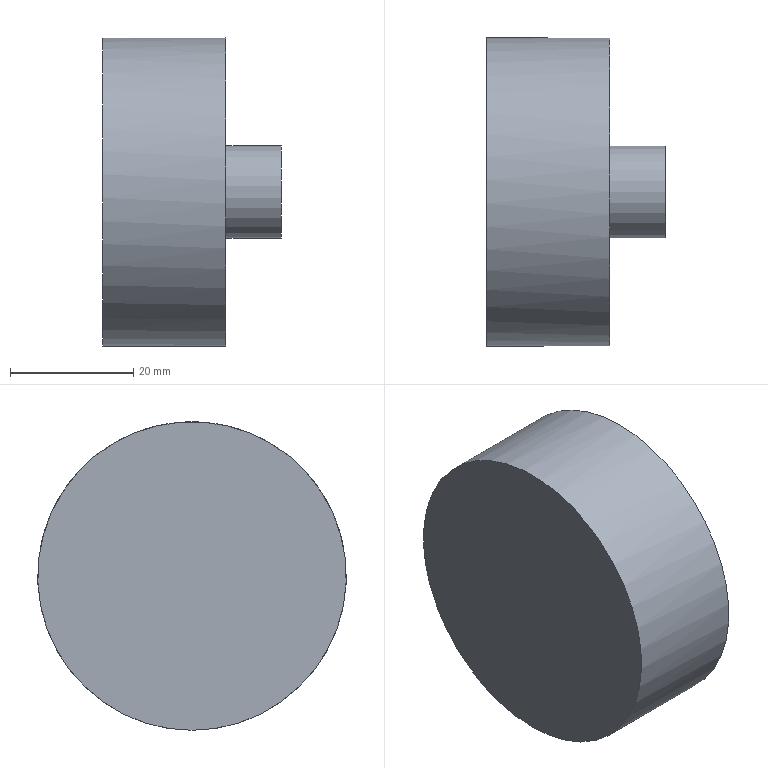Part | STEP file | Tube necking machine_id618_x_t | 1 solid | 5 faces | box 29 x 50 x 50 mm | volume 40860 mm3 | plane 3 | cylinder 2 | commonest cylinder face diameters 15 x1 50 x1
STEP:
#1=CARTESIAN_POINT('',(0.,0.,0.));
#2=DIRECTION('',(0.,0.,1.));
#3=DIRECTION('',(1.,0.,0.));
#4=AXIS2_PLACEMENT_3D('',#1,#2,#3);
#5=CARTESIAN_POINT('',(270.5,50.,197.5));
#6=VERTEX_POINT('',#5);
#7=CARTESIAN_POINT('',(270.5,50.,182.5));
#8=VERTEX_POINT('',#7);
#9=CARTESIAN_POINT('',(270.5,50.,190.));
#10=DIRECTION('',(1.,0.,0.));
#11=DIRECTION('',(0.,0.,1.));
#12=AXIS2_PLACEMENT_3D('',#9,#10,#11);
#13=CIRCLE('',#12,7.5);
#14=CARTESIAN_POINT('',(274.5,50.,190.));
#15=DIRECTION('',(1.,0.,0.));
#16=DIRECTION('',(0.,0.,-1.));
#17=AXIS2_PLACEMENT_3D('',#14,#15,#16);
#18=CYLINDRICAL_SURFACE('',#17,7.5);
#19=CARTESIAN_POINT('',(3.142,-4.));
#20=DIRECTION('',(1.,0.));
#21=VECTOR('',#20,1.);
#22=LINE('',#19,#21);
#23=(GEOMETRIC_REPRESENTATION_CONTEXT(2)PARAMETRIC_REPRESENTATION_CONTEXT()REPRESENTATION_CONTEXT('',''));
#24=DEFINITIONAL_REPRESENTATION('',(#22),#23);
#25=PCURVE('',#18,#24);
#26=CARTESIAN_POINT('',(270.5,50.,190.));
#27=DIRECTION('',(-1.,0.,0.));
#28=DIRECTION('',(0.,0.,1.));
#29=AXIS2_PLACEMENT_3D('',#26,#27,#28);
#30=PLANE('',#29);
#31=CARTESIAN_POINT('',(7.5,0.));
#32=CARTESIAN_POINT('',(7.5,-12.99));
#33=CARTESIAN_POINT('',(-3.75,-6.495));
#34=CARTESIAN_POINT('',(-15.,0.));
#35=CARTESIAN_POINT('',(-3.75,6.495));
#36=CARTESIAN_POINT('',(7.5,12.99));
#37=CARTESIAN_POINT('',(7.5,0.));
#38=(BOUNDED_CURVE()B_SPLINE_CURVE(2,(#31,#32,#33,#34,#35,#36,#37),.UNSPECIFIED.,.T.,.F.)B_SPLINE_CURVE_WITH_KNOTS((1,2,2,2,2,1),(-2.094,0.,2.094,4.189,6.283,8.378),.UNSPECIFIED.)CURVE()GEOMETRIC_REPRESENTATION_ITEM()RATIONAL_B_SPLINE_CURVE((1.,0.5,1.,0.5,1.,0.5,1.))REPRESENTATION_ITEM(''));
#39=(GEOMETRIC_REPRESENTATION_CONTEXT(2)PARAMETRIC_REPRESENTATION_CONTEXT()REPRESENTATION_CONTEXT('',''));
#40=DEFINITIONAL_REPRESENTATION('',(#38),#39);
#41=PCURVE('',#30,#40);
#42=SURFACE_CURVE('',#13,(#25,#41),.PCURVE_S1.);
#43=EDGE_CURVE('',#6,#8,#42,.T.);
#44=ORIENTED_EDGE('',*,*,#43,.T.);
#45=CARTESIAN_POINT('',(279.5,50.,182.5));
#46=VERTEX_POINT('',#45);
#47=CARTESIAN_POINT('',(270.5,50.,182.5));
#48=CARTESIAN_POINT('',(279.5,50.,182.5));
#49=B_SPLINE_CURVE_WITH_KNOTS('',1,(#47,#48),.UNSPECIFIED.,.F.,.F.,(2,2),(-4.,5.),.PIECEWISE_BEZIER_KNOTS.);
#50=CARTESIAN_POINT('',(6.283,0.));
#51=DIRECTION('',(0.,1.));
#52=VECTOR('',#51,1.);
#53=LINE('',#50,#52);
#54=(GEOMETRIC_REPRESENTATION_CONTEXT(2)PARAMETRIC_REPRESENTATION_CONTEXT()REPRESENTATION_CONTEXT('',''));
#55=DEFINITIONAL_REPRESENTATION('',(#53),#54);
#56=PCURVE('',#18,#55);
#57=CARTESIAN_POINT('',(0.,0.));
#58=DIRECTION('',(0.,1.));
#59=VECTOR('',#58,1.);
#60=LINE('',#57,#59);
#61=(GEOMETRIC_REPRESENTATION_CONTEXT(2)PARAMETRIC_REPRESENTATION_CONTEXT()REPRESENTATION_CONTEXT('',''));
#62=DEFINITIONAL_REPRESENTATION('',(#60),#61);
#63=PCURVE('',#18,#62);
#64=SEAM_CURVE('',#49,(#56,#63),.PCURVE_S1.);
#65=EDGE_CURVE('',#8,#46,#64,.T.);
#66=ORIENTED_EDGE('',*,*,#65,.T.);
#67=CARTESIAN_POINT('',(279.5,50.,190.));
#68=DIRECTION('',(1.,0.,0.));
#69=DIRECTION('',(0.,0.,-1.));
#70=AXIS2_PLACEMENT_3D('',#67,#68,#69);
#71=CIRCLE('',#70,7.5);
#72=CARTESIAN_POINT('',(0.,5.));
#73=DIRECTION('',(1.,0.));
#74=VECTOR('',#73,1.);
#75=LINE('',#72,#74);
#76=(GEOMETRIC_REPRESENTATION_CONTEXT(2)PARAMETRIC_REPRESENTATION_CONTEXT()REPRESENTATION_CONTEXT('',''));
#77=DEFINITIONAL_REPRESENTATION('',(#75),#76);
#78=PCURVE('',#18,#77);
#79=CARTESIAN_POINT('',(279.5,50.,190.));
#80=DIRECTION('',(1.,0.,0.));
#81=DIRECTION('',(0.,0.,-1.));
#82=AXIS2_PLACEMENT_3D('',#79,#80,#81);
#83=PLANE('',#82);
#84=CARTESIAN_POINT('',(0.,0.));
#85=DIRECTION('',(1.,0.));
#86=AXIS2_PLACEMENT_2D('',#84,#85);
#87=CIRCLE('',#86,7.5);
#88=(GEOMETRIC_REPRESENTATION_CONTEXT(2)PARAMETRIC_REPRESENTATION_CONTEXT()REPRESENTATION_CONTEXT('',''));
#89=DEFINITIONAL_REPRESENTATION('',(#87),#88);
#90=PCURVE('',#83,#89);
#91=SURFACE_CURVE('',#71,(#78,#90),.PCURVE_S1.);
#92=EDGE_CURVE('',#46,#46,#91,.T.);
#93=ORIENTED_EDGE('',*,*,#92,.F.);
#94=ORIENTED_EDGE('',*,*,#65,.F.);
#95=CARTESIAN_POINT('',(270.5,50.,190.));
#96=DIRECTION('',(1.,0.,0.));
#97=DIRECTION('',(0.,0.,1.));
#98=AXIS2_PLACEMENT_3D('',#95,#96,#97);
#99=CIRCLE('',#98,7.5);
#100=CARTESIAN_POINT('',(-3.142,-4.));
#101=DIRECTION('',(1.,0.));
#102=VECTOR('',#101,1.);
#103=LINE('',#100,#102);
#104=(GEOMETRIC_REPRESENTATION_CONTEXT(2)PARAMETRIC_REPRESENTATION_CONTEXT()REPRESENTATION_CONTEXT('',''));
#105=DEFINITIONAL_REPRESENTATION('',(#103),#104);
#106=PCURVE('',#18,#105);
#107=CARTESIAN_POINT('',(7.5,0.));
#108=CARTESIAN_POINT('',(7.5,-12.99));
#109=CARTESIAN_POINT('',(-3.75,-6.495));
#110=CARTESIAN_POINT('',(-15.,0.));
#111=CARTESIAN_POINT('',(-3.75,6.495));
#112=CARTESIAN_POINT('',(7.5,12.99));
#113=CARTESIAN_POINT('',(7.5,0.));
#114=(BOUNDED_CURVE()B_SPLINE_CURVE(2,(#107,#108,#109,#110,#111,#112,#113),.UNSPECIFIED.,.T.,.F.)B_SPLINE_CURVE_WITH_KNOTS((1,2,2,2,2,1),(-2.094,0.,2.094,4.189,6.283,8.378),.UNSPECIFIED.)CURVE()GEOMETRIC_REPRESENTATION_ITEM()RATIONAL_B_SPLINE_CURVE((1.,0.5,1.,0.5,1.,0.5,1.))REPRESENTATION_ITEM(''));
#115=(GEOMETRIC_REPRESENTATION_CONTEXT(2)PARAMETRIC_REPRESENTATION_CONTEXT()REPRESENTATION_CONTEXT('',''));
#116=DEFINITIONAL_REPRESENTATION('',(#114),#115);
#117=PCURVE('',#30,#116);
#118=SURFACE_CURVE('',#99,(#106,#117),.PCURVE_S1.);
#119=EDGE_CURVE('',#8,#6,#118,.T.);
#120=ORIENTED_EDGE('',*,*,#119,.T.);
#121=EDGE_LOOP('',(#44,#66,#93,#94,#120));
#122=FACE_BOUND('',#121,.T.);
#123=ADVANCED_FACE('',(#122),#18,.T.);
#124=ORIENTED_EDGE('',*,*,#92,.T.);
#125=EDGE_LOOP('',(#124));
#126=FACE_BOUND('',#125,.T.);
#127=ADVANCED_FACE('',(#126),#83,.T.);
#128=CARTESIAN_POINT('',(250.5,50.,165.));
#129=VERTEX_POINT('',#128);
#130=CARTESIAN_POINT('',(250.5,50.,190.));
#131=DIRECTION('',(1.,0.,0.));
#132=DIRECTION('',(0.,0.,-1.));
#133=AXIS2_PLACEMENT_3D('',#130,#131,#132);
#134=CIRCLE('',#133,25.);
#135=CARTESIAN_POINT('',(250.5,80.,332.));
#136=DIRECTION('',(1.,0.,0.));
#137=DIRECTION('',(0.,0.,-1.));
#138=AXIS2_PLACEMENT_3D('',#135,#136,#137);
#139=PLANE('',#138);
#140=CARTESIAN_POINT('',(142.,-30.));
#141=DIRECTION('',(1.,0.));
#142=AXIS2_PLACEMENT_2D('',#140,#141);
#143=CIRCLE('',#142,25.);
#144=(GEOMETRIC_REPRESENTATION_CONTEXT(2)PARAMETRIC_REPRESENTATION_CONTEXT()REPRESENTATION_CONTEXT('',''));
#145=DEFINITIONAL_REPRESENTATION('',(#143),#144);
#146=PCURVE('',#139,#145);
#147=CARTESIAN_POINT('',(36.9,50.,190.));
#148=DIRECTION('',(1.,0.,0.));
#149=DIRECTION('',(0.,0.,-1.));
#150=AXIS2_PLACEMENT_3D('',#147,#148,#149);
#151=CYLINDRICAL_SURFACE('',#150,25.);
#152=CARTESIAN_POINT('',(0.,213.6));
#153=DIRECTION('',(1.,0.));
#154=VECTOR('',#153,1.);
#155=LINE('',#152,#154);
#156=(GEOMETRIC_REPRESENTATION_CONTEXT(2)PARAMETRIC_REPRESENTATION_CONTEXT()REPRESENTATION_CONTEXT('',''));
#157=DEFINITIONAL_REPRESENTATION('',(#155),#156);
#158=PCURVE('',#151,#157);
#159=SURFACE_CURVE('',#134,(#146,#158),.PCURVE_S1.);
#160=EDGE_CURVE('',#129,#129,#159,.T.);
#161=ORIENTED_EDGE('',*,*,#160,.F.);
#162=EDGE_LOOP('',(#161));
#163=FACE_BOUND('',#162,.T.);
#164=ADVANCED_FACE('',(#163),#139,.F.);
#165=ORIENTED_EDGE('',*,*,#43,.F.);
#166=ORIENTED_EDGE('',*,*,#119,.F.);
#167=EDGE_LOOP('',(#165,#166));
#168=FACE_BOUND('',#167,.T.);
#169=CARTESIAN_POINT('',(270.5,50.,215.));
#170=VERTEX_POINT('',#169);
#171=CARTESIAN_POINT('',(270.5,50.,165.));
#172=VERTEX_POINT('',#171);
#173=CARTESIAN_POINT('',(270.5,50.,190.));
#174=DIRECTION('',(-1.,0.,0.));
#175=DIRECTION('',(0.,0.,1.));
#176=AXIS2_PLACEMENT_3D('',#173,#174,#175);
#177=CIRCLE('',#176,25.);
#178=CARTESIAN_POINT('',(0.,0.));
#179=DIRECTION('',(1.,0.));
#180=AXIS2_PLACEMENT_2D('',#178,#179);
#181=CIRCLE('',#180,25.);
#182=(GEOMETRIC_REPRESENTATION_CONTEXT(2)PARAMETRIC_REPRESENTATION_CONTEXT()REPRESENTATION_CONTEXT('',''));
#183=DEFINITIONAL_REPRESENTATION('',(#181),#182);
#184=PCURVE('',#30,#183);
#185=CARTESIAN_POINT('',(3.142,233.6));
#186=DIRECTION('',(-1.,0.));
#187=VECTOR('',#186,1.);
#188=LINE('',#185,#187);
#189=(GEOMETRIC_REPRESENTATION_CONTEXT(2)PARAMETRIC_REPRESENTATION_CONTEXT()REPRESENTATION_CONTEXT('',''));
#190=DEFINITIONAL_REPRESENTATION('',(#188),#189);
#191=PCURVE('',#151,#190);
#192=SURFACE_CURVE('',#177,(#184,#191),.PCURVE_S1.);
#193=EDGE_CURVE('',#170,#172,#192,.T.);
#194=ORIENTED_EDGE('',*,*,#193,.F.);
#195=CARTESIAN_POINT('',(270.5,50.,190.));
#196=DIRECTION('',(-1.,0.,0.));
#197=DIRECTION('',(0.,0.,1.));
#198=AXIS2_PLACEMENT_3D('',#195,#196,#197);
#199=CIRCLE('',#198,25.);
#200=CARTESIAN_POINT('',(0.,0.));
#201=DIRECTION('',(1.,0.));
#202=AXIS2_PLACEMENT_2D('',#200,#201);
#203=CIRCLE('',#202,25.);
#204=(GEOMETRIC_REPRESENTATION_CONTEXT(2)PARAMETRIC_REPRESENTATION_CONTEXT()REPRESENTATION_CONTEXT('',''));
#205=DEFINITIONAL_REPRESENTATION('',(#203),#204);
#206=PCURVE('',#30,#205);
#207=CARTESIAN_POINT('',(9.425,233.6));
#208=DIRECTION('',(-1.,0.));
#209=VECTOR('',#208,1.);
#210=LINE('',#207,#209);
#211=(GEOMETRIC_REPRESENTATION_CONTEXT(2)PARAMETRIC_REPRESENTATION_CONTEXT()REPRESENTATION_CONTEXT('',''));
#212=DEFINITIONAL_REPRESENTATION('',(#210),#211);
#213=PCURVE('',#151,#212);
#214=SURFACE_CURVE('',#199,(#206,#213),.PCURVE_S1.);
#215=EDGE_CURVE('',#172,#170,#214,.T.);
#216=ORIENTED_EDGE('',*,*,#215,.F.);
#217=EDGE_LOOP('',(#194,#216));
#218=FACE_BOUND('',#217,.T.);
#219=ADVANCED_FACE('',(#168,#218),#30,.F.);
#220=ORIENTED_EDGE('',*,*,#160,.T.);
#221=CARTESIAN_POINT('',(250.5,50.,165.));
#222=CARTESIAN_POINT('',(270.5,50.,165.));
#223=B_SPLINE_CURVE_WITH_KNOTS('',1,(#221,#222),.UNSPECIFIED.,.F.,.F.,(2,2),(213.6,233.6),.PIECEWISE_BEZIER_KNOTS.);
#224=CARTESIAN_POINT('',(6.283,0.));
#225=DIRECTION('',(0.,1.));
#226=VECTOR('',#225,1.);
#227=LINE('',#224,#226);
#228=(GEOMETRIC_REPRESENTATION_CONTEXT(2)PARAMETRIC_REPRESENTATION_CONTEXT()REPRESENTATION_CONTEXT('',''));
#229=DEFINITIONAL_REPRESENTATION('',(#227),#228);
#230=PCURVE('',#151,#229);
#231=CARTESIAN_POINT('',(0.,0.));
#232=DIRECTION('',(0.,1.));
#233=VECTOR('',#232,1.);
#234=LINE('',#231,#233);
#235=(GEOMETRIC_REPRESENTATION_CONTEXT(2)PARAMETRIC_REPRESENTATION_CONTEXT()REPRESENTATION_CONTEXT('',''));
#236=DEFINITIONAL_REPRESENTATION('',(#234),#235);
#237=PCURVE('',#151,#236);
#238=SEAM_CURVE('',#223,(#230,#237),.PCURVE_S1.);
#239=EDGE_CURVE('',#129,#172,#238,.T.);
#240=ORIENTED_EDGE('',*,*,#239,.T.);
#241=ORIENTED_EDGE('',*,*,#215,.T.);
#242=ORIENTED_EDGE('',*,*,#193,.T.);
#243=ORIENTED_EDGE('',*,*,#239,.F.);
#244=EDGE_LOOP('',(#220,#240,#241,#242,#243));
#245=FACE_BOUND('',#244,.T.);
#246=ADVANCED_FACE('',(#245),#151,.T.);
#247=CLOSED_SHELL('',(#123,#127,#164,#219,#246));
#248=MANIFOLD_SOLID_BREP('',#247);
#249=(LENGTH_UNIT()NAMED_UNIT(*)SI_UNIT(.MILLI.,.METRE.));
#250=UNCERTAINTY_MEASURE_WITH_UNIT(LENGTH_MEASURE(0.000005),#249,'','');
#251=(NAMED_UNIT(*)PLANE_ANGLE_UNIT()SI_UNIT($,.RADIAN.));
#252=(NAMED_UNIT(*)SI_UNIT($,.STERADIAN.)SOLID_ANGLE_UNIT());
#253=(GEOMETRIC_REPRESENTATION_CONTEXT(3)GLOBAL_UNCERTAINTY_ASSIGNED_CONTEXT((#250))GLOBAL_UNIT_ASSIGNED_CONTEXT((#249,#251,#252))REPRESENTATION_CONTEXT('',''));
#254=ADVANCED_BREP_SHAPE_REPRESENTATION('',(#4,#248),#253);